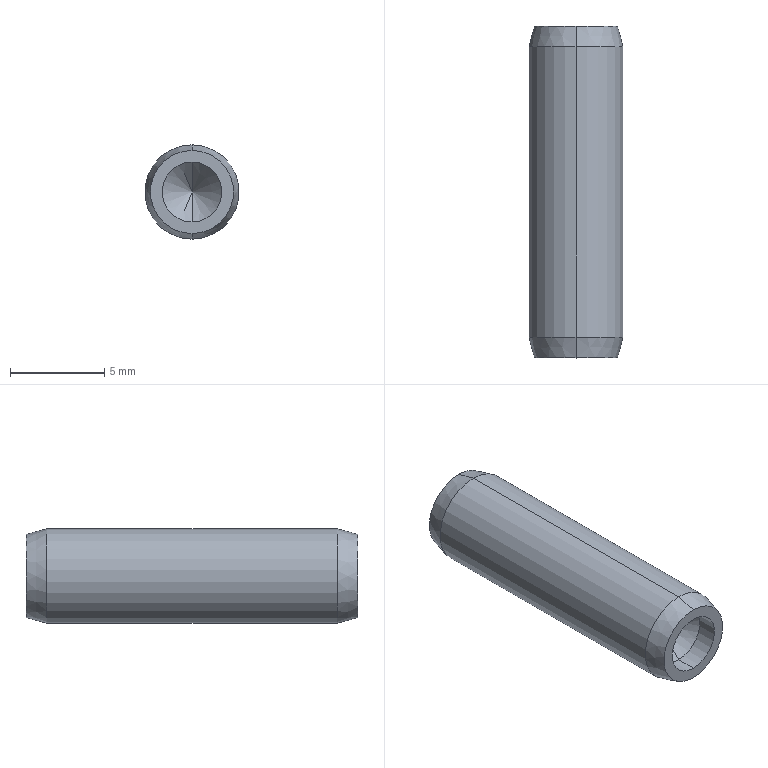Part | STEP file | 1 solid | 25 faces | box 5 x 17.6 x 5 mm | volume 315.252 mm3 | cone 10 | plane 9 | cylinder 6 | commonest cylinder face diameters 1.95 x2 3.175 x2 5 x2
STEP:
#1=CARTESIAN_POINT('',(0.,14.1,-0.975));
#2=VERTEX_POINT('',#1);
#3=CARTESIAN_POINT('',(0.,14.6,-0.975));
#4=VERTEX_POINT('',#3);
#5=CARTESIAN_POINT('',(0.,17.6,-0.975));
#6=DIRECTION('',(0.,1.,0.));
#7=VECTOR('',#6,1000.);
#8=LINE('',#5,#7);
#9=EDGE_CURVE('',#2,#4,#8,.T.);
#10=ORIENTED_EDGE('',*,*,#9,.F.);
#11=CARTESIAN_POINT('',(0.,14.1,0.975));
#12=VERTEX_POINT('',#11);
#13=CARTESIAN_POINT('',(0.,14.1,0.));
#14=DIRECTION('',(0.,1.,0.));
#15=DIRECTION('',(0.,0.,1.));
#16=AXIS2_PLACEMENT_3D('',#13,#14,#15);
#17=CIRCLE('',#16,0.975);
#18=EDGE_CURVE('',#12,#2,#17,.T.);
#19=ORIENTED_EDGE('',*,*,#18,.F.);
#20=CARTESIAN_POINT('',(0.,14.6,0.975));
#21=VERTEX_POINT('',#20);
#22=CARTESIAN_POINT('',(0.,17.6,0.975));
#23=DIRECTION('',(0.,1.,0.));
#24=VECTOR('',#23,1000.);
#25=LINE('',#22,#24);
#26=EDGE_CURVE('',#12,#21,#25,.T.);
#27=ORIENTED_EDGE('',*,*,#26,.T.);
#28=CARTESIAN_POINT('',(0.,14.6,0.));
#29=DIRECTION('',(0.,-1.,0.));
#30=DIRECTION('',(0.,0.,1.));
#31=AXIS2_PLACEMENT_3D('',#28,#29,#30);
#32=CIRCLE('',#31,0.975);
#33=EDGE_CURVE('',#4,#21,#32,.T.);
#34=ORIENTED_EDGE('',*,*,#33,.F.);
#35=EDGE_LOOP('',(#10,#19,#27,#34));
#36=FACE_OUTER_BOUND('',#35,.T.);
#37=CARTESIAN_POINT('',(0.,17.6,0.));
#38=DIRECTION('',(0.,1.,0.));
#39=DIRECTION('',(0.,0.,1.));
#40=AXIS2_PLACEMENT_3D('',#37,#38,#39);
#41=CYLINDRICAL_SURFACE('',#40,0.975);
#42=ADVANCED_FACE('',(#36),#41,.F.);
#43=CARTESIAN_POINT('',(0.,13.514,0.));
#44=VERTEX_POINT('',#43);
#45=CARTESIAN_POINT('',(0.,14.1,-0.975));
#46=DIRECTION('',(0.,0.515,-0.8572));
#47=VECTOR('',#46,1000.);
#48=LINE('',#45,#47);
#49=EDGE_CURVE('',#44,#2,#48,.T.);
#50=ORIENTED_EDGE('',*,*,#49,.F.);
#51=CARTESIAN_POINT('',(0.,14.1,0.975));
#52=DIRECTION('',(0.,0.515,0.8572));
#53=VECTOR('',#52,1000.);
#54=LINE('',#51,#53);
#55=EDGE_CURVE('',#44,#12,#54,.T.);
#56=ORIENTED_EDGE('',*,*,#55,.T.);
#57=ORIENTED_EDGE('',*,*,#18,.T.);
#58=EDGE_LOOP('',(#50,#56,#57));
#59=FACE_OUTER_BOUND('',#58,.T.);
#60=CARTESIAN_POINT('',(0.,14.1,0.));
#61=DIRECTION('',(0.,1.,0.));
#62=DIRECTION('',(0.,0.,1.));
#63=AXIS2_PLACEMENT_3D('',#60,#61,#62);
#64=CONICAL_SURFACE('',#63,0.975,1.03);
#65=ADVANCED_FACE('',(#59),#64,.F.);
#66=CARTESIAN_POINT('',(1.155,17.58,0.));
#67=VERTEX_POINT('',#66);
#68=CARTESIAN_POINT('',(0.5774,17.58,-1.));
#69=VERTEX_POINT('',#68);
#70=CARTESIAN_POINT('',(1.155,17.58,0.));
#71=CARTESIAN_POINT('',(1.104,17.529,-0.08728));
#72=CARTESIAN_POINT('',(1.031,17.472,-0.215));
#73=CARTESIAN_POINT('',(0.9596,17.443,-0.338));
#74=CARTESIAN_POINT('',(0.9129,17.429,-0.4189));
#75=CARTESIAN_POINT('',(0.889,17.426,-0.4602));
#76=CARTESIAN_POINT('',(0.7793,17.423,-0.6502));
#77=CARTESIAN_POINT('',(0.6828,17.474,-0.8174));
#78=CARTESIAN_POINT('',(0.5774,17.58,-1.));
#79=B_SPLINE_CURVE_WITH_KNOTS('',3,(#70,#71,#72,#73,#74,#75,#76,#77,#78),.UNSPECIFIED.,.F.,.F.,(4,1,2,2,4),(0.,0.25,0.375,0.5,1.),.UNSPECIFIED.);
#80=EDGE_CURVE('',#67,#69,#79,.T.);
#81=ORIENTED_EDGE('',*,*,#80,.T.);
#82=CARTESIAN_POINT('',(0.5774,14.6,-1.));
#83=VERTEX_POINT('',#82);
#84=CARTESIAN_POINT('',(0.5774,14.6,-1.));
#85=DIRECTION('',(0.,1.,0.));
#86=VECTOR('',#85,1000.);
#87=LINE('',#84,#86);
#88=EDGE_CURVE('',#83,#69,#87,.T.);
#89=ORIENTED_EDGE('',*,*,#88,.F.);
#90=CARTESIAN_POINT('',(1.155,14.6,0.));
#91=VERTEX_POINT('',#90);
#92=CARTESIAN_POINT('',(1.155,14.6,0.));
#93=DIRECTION('',(-0.5,0.,-0.866));
#94=VECTOR('',#93,1000.);
#95=LINE('',#92,#94);
#96=EDGE_CURVE('',#91,#83,#95,.T.);
#97=ORIENTED_EDGE('',*,*,#96,.F.);
#98=CARTESIAN_POINT('',(1.155,14.6,0.));
#99=DIRECTION('',(0.,1.,0.));
#100=VECTOR('',#99,1000.);
#101=LINE('',#98,#100);
#102=EDGE_CURVE('',#91,#67,#101,.T.);
#103=ORIENTED_EDGE('',*,*,#102,.T.);
#104=EDGE_LOOP('',(#81,#89,#97,#103));
#105=FACE_OUTER_BOUND('',#104,.T.);
#106=CARTESIAN_POINT('',(1.155,14.6,0.));
#107=DIRECTION('',(0.866,0.,-0.5));
#108=DIRECTION('',(0.,-1.,0.));
#109=AXIS2_PLACEMENT_3D('',#106,#107,#108);
#110=PLANE('',#109);
#111=ADVANCED_FACE('',(#105),#110,.F.);
#112=CARTESIAN_POINT('',(0.,17.425,-1.));
#113=VERTEX_POINT('',#112);
#114=CARTESIAN_POINT('',(0.5774,17.58,-1.));
#115=CARTESIAN_POINT('',(0.3711,17.477,-1.));
#116=CARTESIAN_POINT('',(0.1786,17.425,-1.));
#117=CARTESIAN_POINT('',(0.,17.425,-1.));
#118=B_SPLINE_CURVE_WITH_KNOTS('',3,(#114,#115,#116,#117),.UNSPECIFIED.,.F.,.F.,(4,4),(0.,1.),.UNSPECIFIED.);
#119=EDGE_CURVE('',#69,#113,#118,.T.);
#120=ORIENTED_EDGE('',*,*,#119,.T.);
#121=CARTESIAN_POINT('',(-0.5774,17.58,-1.));
#122=VERTEX_POINT('',#121);
#123=CARTESIAN_POINT('',(0.,17.425,-1.));
#124=CARTESIAN_POINT('',(-0.1786,17.425,-1.));
#125=CARTESIAN_POINT('',(-0.3711,17.477,-1.));
#126=CARTESIAN_POINT('',(-0.5774,17.58,-1.));
#127=B_SPLINE_CURVE_WITH_KNOTS('',3,(#123,#124,#125,#126),.UNSPECIFIED.,.F.,.F.,(4,4),(0.,1.),.UNSPECIFIED.);
#128=EDGE_CURVE('',#113,#122,#127,.T.);
#129=ORIENTED_EDGE('',*,*,#128,.T.);
#130=CARTESIAN_POINT('',(-0.5774,14.6,-1.));
#131=VERTEX_POINT('',#130);
#132=CARTESIAN_POINT('',(-0.5774,14.6,-1.));
#133=DIRECTION('',(0.,1.,0.));
#134=VECTOR('',#133,1000.);
#135=LINE('',#132,#134);
#136=EDGE_CURVE('',#131,#122,#135,.T.);
#137=ORIENTED_EDGE('',*,*,#136,.F.);
#138=CARTESIAN_POINT('',(0.5774,14.6,-1.));
#139=DIRECTION('',(-1.,0.,0.));
#140=VECTOR('',#139,1000.);
#141=LINE('',#138,#140);
#142=EDGE_CURVE('',#83,#131,#141,.T.);
#143=ORIENTED_EDGE('',*,*,#142,.F.);
#144=ORIENTED_EDGE('',*,*,#88,.T.);
#145=EDGE_LOOP('',(#120,#129,#137,#143,#144));
#146=FACE_OUTER_BOUND('',#145,.T.);
#147=CARTESIAN_POINT('',(0.5774,14.6,-1.));
#148=DIRECTION('',(0.,0.,-1.));
#149=DIRECTION('',(-1.,0.,0.));
#150=AXIS2_PLACEMENT_3D('',#147,#148,#149);
#151=PLANE('',#150);
#152=ADVANCED_FACE('',(#146),#151,.F.);
#153=CARTESIAN_POINT('',(-1.155,17.58,0.));
#154=VERTEX_POINT('',#153);
#155=CARTESIAN_POINT('',(-0.5774,17.58,-1.));
#156=CARTESIAN_POINT('',(-0.6277,17.529,-0.9127));
#157=CARTESIAN_POINT('',(-0.7015,17.472,-0.785));
#158=CARTESIAN_POINT('',(-0.7725,17.443,-0.662));
#159=CARTESIAN_POINT('',(-0.8192,17.429,-0.5811));
#160=CARTESIAN_POINT('',(-0.843,17.426,-0.5398));
#161=CARTESIAN_POINT('',(-0.9527,17.423,-0.3498));
#162=CARTESIAN_POINT('',(-1.049,17.474,-0.1826));
#163=CARTESIAN_POINT('',(-1.155,17.58,0.));
#164=B_SPLINE_CURVE_WITH_KNOTS('',3,(#155,#156,#157,#158,#159,#160,#161,#162,#163),.UNSPECIFIED.,.F.,.F.,(4,1,2,2,4),(0.,0.25,0.375,0.5,1.),.UNSPECIFIED.);
#165=EDGE_CURVE('',#122,#154,#164,.T.);
#166=ORIENTED_EDGE('',*,*,#165,.T.);
#167=CARTESIAN_POINT('',(-1.155,14.6,0.));
#168=VERTEX_POINT('',#167);
#169=CARTESIAN_POINT('',(-1.155,14.6,0.));
#170=DIRECTION('',(0.,1.,0.));
#171=VECTOR('',#170,1000.);
#172=LINE('',#169,#171);
#173=EDGE_CURVE('',#168,#154,#172,.T.);
#174=ORIENTED_EDGE('',*,*,#173,.F.);
#175=CARTESIAN_POINT('',(-0.5774,14.6,-1.));
#176=DIRECTION('',(-0.5,0.,0.866));
#177=VECTOR('',#176,1000.);
#178=LINE('',#175,#177);
#179=EDGE_CURVE('',#131,#168,#178,.T.);
#180=ORIENTED_EDGE('',*,*,#179,.F.);
#181=ORIENTED_EDGE('',*,*,#136,.T.);
#182=EDGE_LOOP('',(#166,#174,#180,#181));
#183=FACE_OUTER_BOUND('',#182,.T.);
#184=CARTESIAN_POINT('',(-0.5774,14.6,-1.));
#185=DIRECTION('',(-0.866,0.,-0.5));
#186=DIRECTION('',(-0.5,0.,0.866));
#187=AXIS2_PLACEMENT_3D('',#184,#185,#186);
#188=PLANE('',#187);
#189=ADVANCED_FACE('',(#183),#188,.F.);
#190=CARTESIAN_POINT('',(-0.5774,17.58,1.));
#191=VERTEX_POINT('',#190);
#192=CARTESIAN_POINT('',(-1.155,17.58,0.));
#193=CARTESIAN_POINT('',(-1.104,17.529,0.08728));
#194=CARTESIAN_POINT('',(-1.031,17.472,0.215));
#195=CARTESIAN_POINT('',(-0.9596,17.443,0.338));
#196=CARTESIAN_POINT('',(-0.9129,17.429,0.4189));
#197=CARTESIAN_POINT('',(-0.889,17.426,0.4602));
#198=CARTESIAN_POINT('',(-0.7793,17.423,0.6502));
#199=CARTESIAN_POINT('',(-0.6828,17.474,0.8174));
#200=CARTESIAN_POINT('',(-0.5774,17.58,1.));
#201=B_SPLINE_CURVE_WITH_KNOTS('',3,(#192,#193,#194,#195,#196,#197,#198,#199,#200),.UNSPECIFIED.,.F.,.F.,(4,1,2,2,4),(0.,0.25,0.375,0.5,1.),.UNSPECIFIED.);
#202=EDGE_CURVE('',#154,#191,#201,.T.);
#203=ORIENTED_EDGE('',*,*,#202,.T.);
#204=CARTESIAN_POINT('',(-0.5774,14.6,1.));
#205=VERTEX_POINT('',#204);
#206=CARTESIAN_POINT('',(-0.5774,14.6,1.));
#207=DIRECTION('',(0.,1.,0.));
#208=VECTOR('',#207,1000.);
#209=LINE('',#206,#208);
#210=EDGE_CURVE('',#205,#191,#209,.T.);
#211=ORIENTED_EDGE('',*,*,#210,.F.);
#212=CARTESIAN_POINT('',(-1.155,14.6,0.));
#213=DIRECTION('',(0.5,0.,0.866));
#214=VECTOR('',#213,1000.);
#215=LINE('',#212,#214);
#216=EDGE_CURVE('',#168,#205,#215,.T.);
#217=ORIENTED_EDGE('',*,*,#216,.F.);
#218=ORIENTED_EDGE('',*,*,#173,.T.);
#219=EDGE_LOOP('',(#203,#211,#217,#218));
#220=FACE_OUTER_BOUND('',#219,.T.);
#221=CARTESIAN_POINT('',(-1.155,14.6,0.));
#222=DIRECTION('',(-0.866,0.,0.5));
#223=DIRECTION('',(0.,1.,0.));
#224=AXIS2_PLACEMENT_3D('',#221,#222,#223);
#225=PLANE('',#224);
#226=ADVANCED_FACE('',(#220),#225,.F.);
#227=CARTESIAN_POINT('',(0.,17.425,1.));
#228=VERTEX_POINT('',#227);
#229=CARTESIAN_POINT('',(-0.5774,17.58,1.));
#230=CARTESIAN_POINT('',(-0.3711,17.477,1.));
#231=CARTESIAN_POINT('',(-0.1786,17.425,1.));
#232=CARTESIAN_POINT('',(0.,17.425,1.));
#233=B_SPLINE_CURVE_WITH_KNOTS('',3,(#229,#230,#231,#232),.UNSPECIFIED.,.F.,.F.,(4,4),(0.,1.),.UNSPECIFIED.);
#234=EDGE_CURVE('',#191,#228,#233,.T.);
#235=ORIENTED_EDGE('',*,*,#234,.T.);
#236=CARTESIAN_POINT('',(0.5774,17.58,1.));
#237=VERTEX_POINT('',#236);
#238=CARTESIAN_POINT('',(0.,17.425,1.));
#239=CARTESIAN_POINT('',(0.1786,17.425,1.));
#240=CARTESIAN_POINT('',(0.3711,17.477,1.));
#241=CARTESIAN_POINT('',(0.5774,17.58,1.));
#242=B_SPLINE_CURVE_WITH_KNOTS('',3,(#238,#239,#240,#241),.UNSPECIFIED.,.F.,.F.,(4,4),(0.,1.),.UNSPECIFIED.);
#243=EDGE_CURVE('',#228,#237,#242,.T.);
#244=ORIENTED_EDGE('',*,*,#243,.T.);
#245=CARTESIAN_POINT('',(0.5774,14.6,1.));
#246=VERTEX_POINT('',#245);
#247=CARTESIAN_POINT('',(0.5774,14.6,1.));
#248=DIRECTION('',(0.,1.,0.));
#249=VECTOR('',#248,1000.);
#250=LINE('',#247,#249);
#251=EDGE_CURVE('',#246,#237,#250,.T.);
#252=ORIENTED_EDGE('',*,*,#251,.F.);
#253=CARTESIAN_POINT('',(-0.5774,14.6,1.));
#254=DIRECTION('',(1.,0.,0.));
#255=VECTOR('',#254,1000.);
#256=LINE('',#253,#255);
#257=EDGE_CURVE('',#205,#246,#256,.T.);
#258=ORIENTED_EDGE('',*,*,#257,.F.);
#259=ORIENTED_EDGE('',*,*,#210,.T.);
#260=EDGE_LOOP('',(#235,#244,#252,#258,#259));
#261=FACE_OUTER_BOUND('',#260,.T.);
#262=CARTESIAN_POINT('',(-0.5774,14.6,1.));
#263=DIRECTION('',(0.,0.,1.));
#264=DIRECTION('',(1.,0.,0.));
#265=AXIS2_PLACEMENT_3D('',#262,#263,#264);
#266=PLANE('',#265);
#267=ADVANCED_FACE('',(#261),#266,.F.);
#268=CARTESIAN_POINT('',(0.5774,17.58,1.));
#269=CARTESIAN_POINT('',(0.6277,17.529,0.9127));
#270=CARTESIAN_POINT('',(0.7015,17.472,0.785));
#271=CARTESIAN_POINT('',(0.7725,17.443,0.662));
#272=CARTESIAN_POINT('',(0.8192,17.429,0.5811));
#273=CARTESIAN_POINT('',(0.843,17.426,0.5398));
#274=CARTESIAN_POINT('',(0.9527,17.423,0.3498));
#275=CARTESIAN_POINT('',(1.049,17.474,0.1826));
#276=CARTESIAN_POINT('',(1.155,17.58,0.));
#277=B_SPLINE_CURVE_WITH_KNOTS('',3,(#268,#269,#270,#271,#272,#273,#274,#275,#276),.UNSPECIFIED.,.F.,.F.,(4,1,2,2,4),(0.,0.25,0.375,0.5,1.),.UNSPECIFIED.);
#278=EDGE_CURVE('',#237,#67,#277,.T.);
#279=ORIENTED_EDGE('',*,*,#278,.T.);
#280=ORIENTED_EDGE('',*,*,#102,.F.);
#281=CARTESIAN_POINT('',(0.5774,14.6,1.));
#282=DIRECTION('',(0.5,0.,-0.866));
#283=VECTOR('',#282,1000.);
#284=LINE('',#281,#283);
#285=EDGE_CURVE('',#246,#91,#284,.T.);
#286=ORIENTED_EDGE('',*,*,#285,.F.);
#287=ORIENTED_EDGE('',*,*,#251,.T.);
#288=EDGE_LOOP('',(#279,#280,#286,#287));
#289=FACE_OUTER_BOUND('',#288,.T.);
#290=CARTESIAN_POINT('',(0.5774,14.6,1.));
#291=DIRECTION('',(0.866,0.,0.5));
#292=DIRECTION('',(0.,-1.,0.));
#293=AXIS2_PLACEMENT_3D('',#290,#291,#292);
#294=PLANE('',#293);
#295=ADVANCED_FACE('',(#289),#294,.F.);
#296=CARTESIAN_POINT('',(0.,14.6,0.));
#297=DIRECTION('',(0.,-1.,0.));
#298=DIRECTION('',(0.,0.,1.));
#299=AXIS2_PLACEMENT_3D('',#296,#297,#298);
#300=CIRCLE('',#299,0.975);
#301=EDGE_CURVE('',#21,#4,#300,.T.);
#302=ORIENTED_EDGE('',*,*,#301,.T.);
#303=ORIENTED_EDGE('',*,*,#33,.T.);
#304=EDGE_LOOP('',(#302,#303));
#305=FACE_BOUND('',#304,.T.);
#306=ORIENTED_EDGE('',*,*,#285,.T.);
#307=ORIENTED_EDGE('',*,*,#96,.T.);
#308=ORIENTED_EDGE('',*,*,#142,.T.);
#309=ORIENTED_EDGE('',*,*,#179,.T.);
#310=ORIENTED_EDGE('',*,*,#216,.T.);
#311=ORIENTED_EDGE('',*,*,#257,.T.);
#312=EDGE_LOOP('',(#306,#307,#308,#309,#310,#311));
#313=FACE_OUTER_BOUND('',#312,.T.);
#314=CARTESIAN_POINT('',(0.,14.6,0.));
#315=DIRECTION('',(0.,1.,0.));
#316=DIRECTION('',(1.,0.,0.));
#317=AXIS2_PLACEMENT_3D('',#314,#315,#316);
#318=PLANE('',#317);
#319=ADVANCED_FACE('',(#305,#313),#318,.T.);
#320=CARTESIAN_POINT('',(0.,17.6,-1.175));
#321=VERTEX_POINT('',#320);
#322=CARTESIAN_POINT('',(0.,17.4,-0.975));
#323=DIRECTION('',(0.,0.7071,-0.7071));
#324=VECTOR('',#323,1000.);
#325=LINE('',#322,#324);
#326=EDGE_CURVE('',#113,#321,#325,.T.);
#327=ORIENTED_EDGE('',*,*,#326,.F.);
#328=ORIENTED_EDGE('',*,*,#119,.F.);
#329=ORIENTED_EDGE('',*,*,#80,.F.);
#330=ORIENTED_EDGE('',*,*,#278,.F.);
#331=ORIENTED_EDGE('',*,*,#243,.F.);
#332=CARTESIAN_POINT('',(0.,17.6,1.175));
#333=VERTEX_POINT('',#332);
#334=CARTESIAN_POINT('',(0.,17.4,0.975));
#335=DIRECTION('',(0.,0.7071,0.7071));
#336=VECTOR('',#335,1000.);
#337=LINE('',#334,#336);
#338=EDGE_CURVE('',#228,#333,#337,.T.);
#339=ORIENTED_EDGE('',*,*,#338,.T.);
#340=CARTESIAN_POINT('',(0.,17.6,0.));
#341=DIRECTION('',(0.,-1.,0.));
#342=DIRECTION('',(0.,0.,1.));
#343=AXIS2_PLACEMENT_3D('',#340,#341,#342);
#344=CIRCLE('',#343,1.175);
#345=EDGE_CURVE('',#321,#333,#344,.T.);
#346=ORIENTED_EDGE('',*,*,#345,.F.);
#347=EDGE_LOOP('',(#327,#328,#329,#330,#331,#339,#346));
#348=FACE_OUTER_BOUND('',#347,.T.);
#349=CARTESIAN_POINT('',(0.,17.4,0.));
#350=DIRECTION('',(0.,1.,0.));
#351=DIRECTION('',(0.,0.,1.));
#352=AXIS2_PLACEMENT_3D('',#349,#350,#351);
#353=CONICAL_SURFACE('',#352,0.975,0.7854);
#354=ADVANCED_FACE('',(#348),#353,.F.);
#355=CARTESIAN_POINT('',(0.,2.688,0.));
#356=VERTEX_POINT('',#355);
#357=CARTESIAN_POINT('',(0.,1.1,1.587));
#358=VERTEX_POINT('',#357);
#359=CARTESIAN_POINT('',(0.,2.688,0.));
#360=DIRECTION('',(0.,-0.7071,0.7071));
#361=VECTOR('',#360,1000.);
#362=LINE('',#359,#361);
#363=EDGE_CURVE('',#356,#358,#362,.T.);
#364=ORIENTED_EDGE('',*,*,#363,.F.);
#365=CARTESIAN_POINT('',(0.,1.1,-1.587));
#366=VERTEX_POINT('',#365);
#367=CARTESIAN_POINT('',(0.,2.688,0.));
#368=DIRECTION('',(0.,-0.7071,-0.7071));
#369=VECTOR('',#368,1000.);
#370=LINE('',#367,#369);
#371=EDGE_CURVE('',#356,#366,#370,.T.);
#372=ORIENTED_EDGE('',*,*,#371,.T.);
#373=CARTESIAN_POINT('',(0.,1.1,0.));
#374=DIRECTION('',(0.,-1.,0.));
#375=DIRECTION('',(0.,0.,-1.));
#376=AXIS2_PLACEMENT_3D('',#373,#374,#375);
#377=CIRCLE('',#376,1.587);
#378=EDGE_CURVE('',#366,#358,#377,.T.);
#379=ORIENTED_EDGE('',*,*,#378,.T.);
#380=EDGE_LOOP('',(#364,#372,#379));
#381=FACE_OUTER_BOUND('',#380,.T.);
#382=CARTESIAN_POINT('',(0.,-997.312,0.));
#383=DIRECTION('',(0.,-1.,0.));
#384=DIRECTION('',(0.,0.,-1.));
#385=AXIS2_PLACEMENT_3D('',#382,#383,#384);
#386=CONICAL_SURFACE('',#385,1000.,0.7854);
#387=ADVANCED_FACE('',(#381),#386,.F.);
#388=CARTESIAN_POINT('',(0.,0.,1.587));
#389=VERTEX_POINT('',#388);
#390=CARTESIAN_POINT('',(0.,0.,1.587));
#391=DIRECTION('',(0.,-1.,0.));
#392=VECTOR('',#391,1000.);
#393=LINE('',#390,#392);
#394=EDGE_CURVE('',#358,#389,#393,.T.);
#395=ORIENTED_EDGE('',*,*,#394,.F.);
#396=ORIENTED_EDGE('',*,*,#378,.F.);
#397=CARTESIAN_POINT('',(0.,0.,-1.587));
#398=VERTEX_POINT('',#397);
#399=CARTESIAN_POINT('',(0.,0.,-1.587));
#400=DIRECTION('',(0.,-1.,0.));
#401=VECTOR('',#400,1000.);
#402=LINE('',#399,#401);
#403=EDGE_CURVE('',#366,#398,#402,.T.);
#404=ORIENTED_EDGE('',*,*,#403,.T.);
#405=CARTESIAN_POINT('',(0.,0.,0.));
#406=DIRECTION('',(0.,-1.,0.));
#407=DIRECTION('',(0.,0.,-1.));
#408=AXIS2_PLACEMENT_3D('',#405,#406,#407);
#409=CIRCLE('',#408,1.587);
#410=EDGE_CURVE('',#398,#389,#409,.T.);
#411=ORIENTED_EDGE('',*,*,#410,.T.);
#412=EDGE_LOOP('',(#395,#396,#404,#411));
#413=FACE_OUTER_BOUND('',#412,.T.);
#414=CARTESIAN_POINT('',(0.,0.,0.));
#415=DIRECTION('',(0.,-1.,0.));
#416=DIRECTION('',(0.,0.,-1.));
#417=AXIS2_PLACEMENT_3D('',#414,#415,#416);
#418=CYLINDRICAL_SURFACE('',#417,1.587);
#419=ADVANCED_FACE('',(#413),#418,.F.);
#420=CARTESIAN_POINT('',(0.,0.,-2.205));
#421=VERTEX_POINT('',#420);
#422=CARTESIAN_POINT('',(0.,1.1,-2.5));
#423=VERTEX_POINT('',#422);
#424=CARTESIAN_POINT('',(0.,1.1,-2.5));
#425=DIRECTION('',(0.,0.9659,-0.2588));
#426=VECTOR('',#425,1000.);
#427=LINE('',#424,#426);
#428=EDGE_CURVE('',#421,#423,#427,.T.);
#429=ORIENTED_EDGE('',*,*,#428,.F.);
#430=CARTESIAN_POINT('',(0.,0.,2.205));
#431=VERTEX_POINT('',#430);
#432=CARTESIAN_POINT('',(0.,0.,0.));
#433=DIRECTION('',(0.,-1.,0.));
#434=DIRECTION('',(0.,0.,1.));
#435=AXIS2_PLACEMENT_3D('',#432,#433,#434);
#436=CIRCLE('',#435,2.205);
#437=EDGE_CURVE('',#431,#421,#436,.T.);
#438=ORIENTED_EDGE('',*,*,#437,.F.);
#439=CARTESIAN_POINT('',(0.,1.1,2.5));
#440=VERTEX_POINT('',#439);
#441=CARTESIAN_POINT('',(0.,1.1,2.5));
#442=DIRECTION('',(0.,0.9659,0.2588));
#443=VECTOR('',#442,1000.);
#444=LINE('',#441,#443);
#445=EDGE_CURVE('',#431,#440,#444,.T.);
#446=ORIENTED_EDGE('',*,*,#445,.T.);
#447=CARTESIAN_POINT('',(0.,1.1,0.));
#448=DIRECTION('',(0.,1.,0.));
#449=DIRECTION('',(0.,0.,1.));
#450=AXIS2_PLACEMENT_3D('',#447,#448,#449);
#451=CIRCLE('',#450,2.5);
#452=EDGE_CURVE('',#423,#440,#451,.T.);
#453=ORIENTED_EDGE('',*,*,#452,.F.);
#454=EDGE_LOOP('',(#429,#438,#446,#453));
#455=FACE_OUTER_BOUND('',#454,.T.);
#456=CARTESIAN_POINT('',(0.,1.1,0.));
#457=DIRECTION('',(0.,1.,0.));
#458=DIRECTION('',(0.,0.,1.));
#459=AXIS2_PLACEMENT_3D('',#456,#457,#458);
#460=CONICAL_SURFACE('',#459,2.5,0.2618);
#461=ADVANCED_FACE('',(#455),#460,.T.);
#462=CARTESIAN_POINT('',(0.,17.6,2.205));
#463=VERTEX_POINT('',#462);
#464=CARTESIAN_POINT('',(0.,16.5,2.5));
#465=VERTEX_POINT('',#464);
#466=CARTESIAN_POINT('',(0.,17.6,2.205));
#467=DIRECTION('',(0.,-0.9659,0.2588));
#468=VECTOR('',#467,1000.);
#469=LINE('',#466,#468);
#470=EDGE_CURVE('',#463,#465,#469,.T.);
#471=ORIENTED_EDGE('',*,*,#470,.F.);
#472=CARTESIAN_POINT('',(0.,17.6,-2.205));
#473=VERTEX_POINT('',#472);
#474=CARTESIAN_POINT('',(0.,17.6,0.));
#475=DIRECTION('',(0.,1.,0.));
#476=DIRECTION('',(0.,0.,1.));
#477=AXIS2_PLACEMENT_3D('',#474,#475,#476);
#478=CIRCLE('',#477,2.205);
#479=EDGE_CURVE('',#473,#463,#478,.T.);
#480=ORIENTED_EDGE('',*,*,#479,.F.);
#481=CARTESIAN_POINT('',(0.,16.5,-2.5));
#482=VERTEX_POINT('',#481);
#483=CARTESIAN_POINT('',(0.,17.6,-2.205));
#484=DIRECTION('',(0.,-0.9659,-0.2588));
#485=VECTOR('',#484,1000.);
#486=LINE('',#483,#485);
#487=EDGE_CURVE('',#473,#482,#486,.T.);
#488=ORIENTED_EDGE('',*,*,#487,.T.);
#489=CARTESIAN_POINT('',(0.,16.5,0.));
#490=DIRECTION('',(0.,-1.,0.));
#491=DIRECTION('',(0.,0.,1.));
#492=AXIS2_PLACEMENT_3D('',#489,#490,#491);
#493=CIRCLE('',#492,2.5);
#494=EDGE_CURVE('',#465,#482,#493,.T.);
#495=ORIENTED_EDGE('',*,*,#494,.F.);
#496=EDGE_LOOP('',(#471,#480,#488,#495));
#497=FACE_OUTER_BOUND('',#496,.T.);
#498=CARTESIAN_POINT('',(0.,17.6,0.));
#499=DIRECTION('',(0.,-1.,0.));
#500=DIRECTION('',(0.,0.,-1.));
#501=AXIS2_PLACEMENT_3D('',#498,#499,#500);
#502=CONICAL_SURFACE('',#501,2.205,0.2618);
#503=ADVANCED_FACE('',(#497),#502,.T.);
#504=ORIENTED_EDGE('',*,*,#410,.F.);
#505=CARTESIAN_POINT('',(0.,0.,0.));
#506=DIRECTION('',(0.,-1.,0.));
#507=DIRECTION('',(0.,0.,-1.));
#508=AXIS2_PLACEMENT_3D('',#505,#506,#507);
#509=CIRCLE('',#508,1.587);
#510=EDGE_CURVE('',#389,#398,#509,.T.);
#511=ORIENTED_EDGE('',*,*,#510,.F.);
#512=EDGE_LOOP('',(#504,#511));
#513=FACE_BOUND('',#512,.T.);
#514=ORIENTED_EDGE('',*,*,#437,.T.);
#515=CARTESIAN_POINT('',(0.,0.,0.));
#516=DIRECTION('',(0.,-1.,0.));
#517=DIRECTION('',(0.,0.,1.));
#518=AXIS2_PLACEMENT_3D('',#515,#516,#517);
#519=CIRCLE('',#518,2.205);
#520=EDGE_CURVE('',#421,#431,#519,.T.);
#521=ORIENTED_EDGE('',*,*,#520,.T.);
#522=EDGE_LOOP('',(#514,#521));
#523=FACE_OUTER_BOUND('',#522,.T.);
#524=CARTESIAN_POINT('',(0.,0.,0.));
#525=DIRECTION('',(0.,1.,0.));
#526=DIRECTION('',(1.,0.,0.));
#527=AXIS2_PLACEMENT_3D('',#524,#525,#526);
#528=PLANE('',#527);
#529=ADVANCED_FACE('',(#513,#523),#528,.F.);
#530=CARTESIAN_POINT('',(0.,17.6,0.));
#531=DIRECTION('',(0.,-1.,0.));
#532=DIRECTION('',(0.,0.,1.));
#533=AXIS2_PLACEMENT_3D('',#530,#531,#532);
#534=CIRCLE('',#533,1.175);
#535=EDGE_CURVE('',#333,#321,#534,.T.);
#536=ORIENTED_EDGE('',*,*,#535,.T.);
#537=ORIENTED_EDGE('',*,*,#345,.T.);
#538=EDGE_LOOP('',(#536,#537));
#539=FACE_BOUND('',#538,.T.);
#540=ORIENTED_EDGE('',*,*,#479,.T.);
#541=CARTESIAN_POINT('',(0.,17.6,0.));
#542=DIRECTION('',(0.,1.,0.));
#543=DIRECTION('',(0.,0.,1.));
#544=AXIS2_PLACEMENT_3D('',#541,#542,#543);
#545=CIRCLE('',#544,2.205);
#546=EDGE_CURVE('',#463,#473,#545,.T.);
#547=ORIENTED_EDGE('',*,*,#546,.T.);
#548=EDGE_LOOP('',(#540,#547));
#549=FACE_OUTER_BOUND('',#548,.T.);
#550=CARTESIAN_POINT('',(0.,17.6,0.));
#551=DIRECTION('',(0.,1.,0.));
#552=DIRECTION('',(1.,0.,0.));
#553=AXIS2_PLACEMENT_3D('',#550,#551,#552);
#554=PLANE('',#553);
#555=ADVANCED_FACE('',(#539,#549),#554,.T.);
#556=CARTESIAN_POINT('',(0.,17.6,2.5));
#557=DIRECTION('',(0.,-1.,0.));
#558=VECTOR('',#557,1000.);
#559=LINE('',#556,#558);
#560=EDGE_CURVE('',#465,#440,#559,.T.);
#561=ORIENTED_EDGE('',*,*,#560,.F.);
#562=ORIENTED_EDGE('',*,*,#494,.T.);
#563=CARTESIAN_POINT('',(0.,17.6,-2.5));
#564=DIRECTION('',(0.,-1.,0.));
#565=VECTOR('',#564,1000.);
#566=LINE('',#563,#565);
#567=EDGE_CURVE('',#482,#423,#566,.T.);
#568=ORIENTED_EDGE('',*,*,#567,.T.);
#569=ORIENTED_EDGE('',*,*,#452,.T.);
#570=EDGE_LOOP('',(#561,#562,#568,#569));
#571=FACE_OUTER_BOUND('',#570,.T.);
#572=CARTESIAN_POINT('',(0.,17.6,0.));
#573=DIRECTION('',(0.,-1.,0.));
#574=DIRECTION('',(0.,0.,-1.));
#575=AXIS2_PLACEMENT_3D('',#572,#573,#574);
#576=CYLINDRICAL_SURFACE('',#575,2.5);
#577=ADVANCED_FACE('',(#571),#576,.T.);
#578=CARTESIAN_POINT('',(0.,16.5,0.));
#579=DIRECTION('',(0.,-1.,0.));
#580=DIRECTION('',(0.,0.,1.));
#581=AXIS2_PLACEMENT_3D('',#578,#579,#580);
#582=CIRCLE('',#581,2.5);
#583=EDGE_CURVE('',#482,#465,#582,.T.);
#584=ORIENTED_EDGE('',*,*,#583,.T.);
#585=ORIENTED_EDGE('',*,*,#560,.T.);
#586=CARTESIAN_POINT('',(0.,1.1,0.));
#587=DIRECTION('',(0.,1.,0.));
#588=DIRECTION('',(0.,0.,1.));
#589=AXIS2_PLACEMENT_3D('',#586,#587,#588);
#590=CIRCLE('',#589,2.5);
#591=EDGE_CURVE('',#440,#423,#590,.T.);
#592=ORIENTED_EDGE('',*,*,#591,.T.);
#593=ORIENTED_EDGE('',*,*,#567,.F.);
#594=EDGE_LOOP('',(#584,#585,#592,#593));
#595=FACE_OUTER_BOUND('',#594,.T.);
#596=CARTESIAN_POINT('',(0.,17.6,0.));
#597=DIRECTION('',(0.,-1.,0.));
#598=DIRECTION('',(0.,0.,-1.));
#599=AXIS2_PLACEMENT_3D('',#596,#597,#598);
#600=CYLINDRICAL_SURFACE('',#599,2.5);
#601=ADVANCED_FACE('',(#595),#600,.T.);
#602=ORIENTED_EDGE('',*,*,#546,.F.);
#603=ORIENTED_EDGE('',*,*,#470,.T.);
#604=ORIENTED_EDGE('',*,*,#583,.F.);
#605=ORIENTED_EDGE('',*,*,#487,.F.);
#606=EDGE_LOOP('',(#602,#603,#604,#605));
#607=FACE_OUTER_BOUND('',#606,.T.);
#608=CARTESIAN_POINT('',(0.,17.6,0.));
#609=DIRECTION('',(0.,-1.,0.));
#610=DIRECTION('',(0.,0.,-1.));
#611=AXIS2_PLACEMENT_3D('',#608,#609,#610);
#612=CONICAL_SURFACE('',#611,2.205,0.2618);
#613=ADVANCED_FACE('',(#607),#612,.T.);
#614=ORIENTED_EDGE('',*,*,#520,.F.);
#615=ORIENTED_EDGE('',*,*,#428,.T.);
#616=ORIENTED_EDGE('',*,*,#591,.F.);
#617=ORIENTED_EDGE('',*,*,#445,.F.);
#618=EDGE_LOOP('',(#614,#615,#616,#617));
#619=FACE_OUTER_BOUND('',#618,.T.);
#620=CARTESIAN_POINT('',(0.,1.1,0.));
#621=DIRECTION('',(0.,1.,0.));
#622=DIRECTION('',(0.,0.,1.));
#623=AXIS2_PLACEMENT_3D('',#620,#621,#622);
#624=CONICAL_SURFACE('',#623,2.5,0.2618);
#625=ADVANCED_FACE('',(#619),#624,.T.);
#626=CARTESIAN_POINT('',(0.,1.1,0.));
#627=DIRECTION('',(0.,-1.,0.));
#628=DIRECTION('',(0.,0.,-1.));
#629=AXIS2_PLACEMENT_3D('',#626,#627,#628);
#630=CIRCLE('',#629,1.587);
#631=EDGE_CURVE('',#358,#366,#630,.T.);
#632=ORIENTED_EDGE('',*,*,#631,.F.);
#633=ORIENTED_EDGE('',*,*,#394,.T.);
#634=ORIENTED_EDGE('',*,*,#510,.T.);
#635=ORIENTED_EDGE('',*,*,#403,.F.);
#636=EDGE_LOOP('',(#632,#633,#634,#635));
#637=FACE_OUTER_BOUND('',#636,.T.);
#638=CARTESIAN_POINT('',(0.,0.,0.));
#639=DIRECTION('',(0.,-1.,0.));
#640=DIRECTION('',(0.,0.,-1.));
#641=AXIS2_PLACEMENT_3D('',#638,#639,#640);
#642=CYLINDRICAL_SURFACE('',#641,1.587);
#643=ADVANCED_FACE('',(#637),#642,.F.);
#644=ORIENTED_EDGE('',*,*,#371,.F.);
#645=ORIENTED_EDGE('',*,*,#363,.T.);
#646=ORIENTED_EDGE('',*,*,#631,.T.);
#647=EDGE_LOOP('',(#644,#645,#646));
#648=FACE_OUTER_BOUND('',#647,.T.);
#649=CARTESIAN_POINT('',(0.,-997.312,0.));
#650=DIRECTION('',(0.,-1.,0.));
#651=DIRECTION('',(0.,0.,-1.));
#652=AXIS2_PLACEMENT_3D('',#649,#650,#651);
#653=CONICAL_SURFACE('',#652,1000.,0.7854);
#654=ADVANCED_FACE('',(#648),#653,.F.);
#655=ORIENTED_EDGE('',*,*,#128,.F.);
#656=ORIENTED_EDGE('',*,*,#326,.T.);
#657=ORIENTED_EDGE('',*,*,#535,.F.);
#658=ORIENTED_EDGE('',*,*,#338,.F.);
#659=ORIENTED_EDGE('',*,*,#234,.F.);
#660=ORIENTED_EDGE('',*,*,#202,.F.);
#661=ORIENTED_EDGE('',*,*,#165,.F.);
#662=EDGE_LOOP('',(#655,#656,#657,#658,#659,#660,#661));
#663=FACE_OUTER_BOUND('',#662,.T.);
#664=CARTESIAN_POINT('',(0.,17.4,0.));
#665=DIRECTION('',(0.,1.,0.));
#666=DIRECTION('',(0.,0.,1.));
#667=AXIS2_PLACEMENT_3D('',#664,#665,#666);
#668=CONICAL_SURFACE('',#667,0.975,0.7854);
#669=ADVANCED_FACE('',(#663),#668,.F.);
#670=ORIENTED_EDGE('',*,*,#55,.F.);
#671=ORIENTED_EDGE('',*,*,#49,.T.);
#672=CARTESIAN_POINT('',(0.,14.1,0.));
#673=DIRECTION('',(0.,1.,0.));
#674=DIRECTION('',(0.,0.,1.));
#675=AXIS2_PLACEMENT_3D('',#672,#673,#674);
#676=CIRCLE('',#675,0.975);
#677=EDGE_CURVE('',#2,#12,#676,.T.);
#678=ORIENTED_EDGE('',*,*,#677,.T.);
#679=EDGE_LOOP('',(#670,#671,#678));
#680=FACE_OUTER_BOUND('',#679,.T.);
#681=CARTESIAN_POINT('',(0.,14.1,0.));
#682=DIRECTION('',(0.,1.,0.));
#683=DIRECTION('',(0.,0.,1.));
#684=AXIS2_PLACEMENT_3D('',#681,#682,#683);
#685=CONICAL_SURFACE('',#684,0.975,1.03);
#686=ADVANCED_FACE('',(#680),#685,.F.);
#687=ORIENTED_EDGE('',*,*,#677,.F.);
#688=ORIENTED_EDGE('',*,*,#9,.T.);
#689=ORIENTED_EDGE('',*,*,#301,.F.);
#690=ORIENTED_EDGE('',*,*,#26,.F.);
#691=EDGE_LOOP('',(#687,#688,#689,#690));
#692=FACE_OUTER_BOUND('',#691,.T.);
#693=CARTESIAN_POINT('',(0.,17.6,0.));
#694=DIRECTION('',(0.,1.,0.));
#695=DIRECTION('',(0.,0.,1.));
#696=AXIS2_PLACEMENT_3D('',#693,#694,#695);
#697=CYLINDRICAL_SURFACE('',#696,0.975);
#698=ADVANCED_FACE('',(#692),#697,.F.);
#699=CLOSED_SHELL('',(#42,#65,#111,#152,#189,#226,#267,#295,#319,#354,#387,#419,#461,#503,#529,#555,#577,#601,#613,#625,#643,#654,#669,#686,#698));
#700=MANIFOLD_SOLID_BREP('',#699);
#701=CARTESIAN_POINT('',(0.,0.,0.));
#702=DIRECTION('',(0.,0.,1.));
#703=DIRECTION('',(1.,0.,0.));
#704=AXIS2_PLACEMENT_3D('',#701,#702,#703);
#705=(LENGTH_UNIT()NAMED_UNIT(*)SI_UNIT(.MILLI.,.METRE.));
#706=UNCERTAINTY_MEASURE_WITH_UNIT(LENGTH_MEASURE(0.00001),#705,'','');
#707=(NAMED_UNIT(*)PLANE_ANGLE_UNIT()SI_UNIT($,.RADIAN.));
#708=(NAMED_UNIT(*)SI_UNIT($,.STERADIAN.)SOLID_ANGLE_UNIT());
#709=(GEOMETRIC_REPRESENTATION_CONTEXT(3)GLOBAL_UNCERTAINTY_ASSIGNED_CONTEXT((#706))GLOBAL_UNIT_ASSIGNED_CONTEXT((#705,#707,#708))REPRESENTATION_CONTEXT('',''));
#710=ADVANCED_BREP_SHAPE_REPRESENTATION('',(#700,#704),#709);